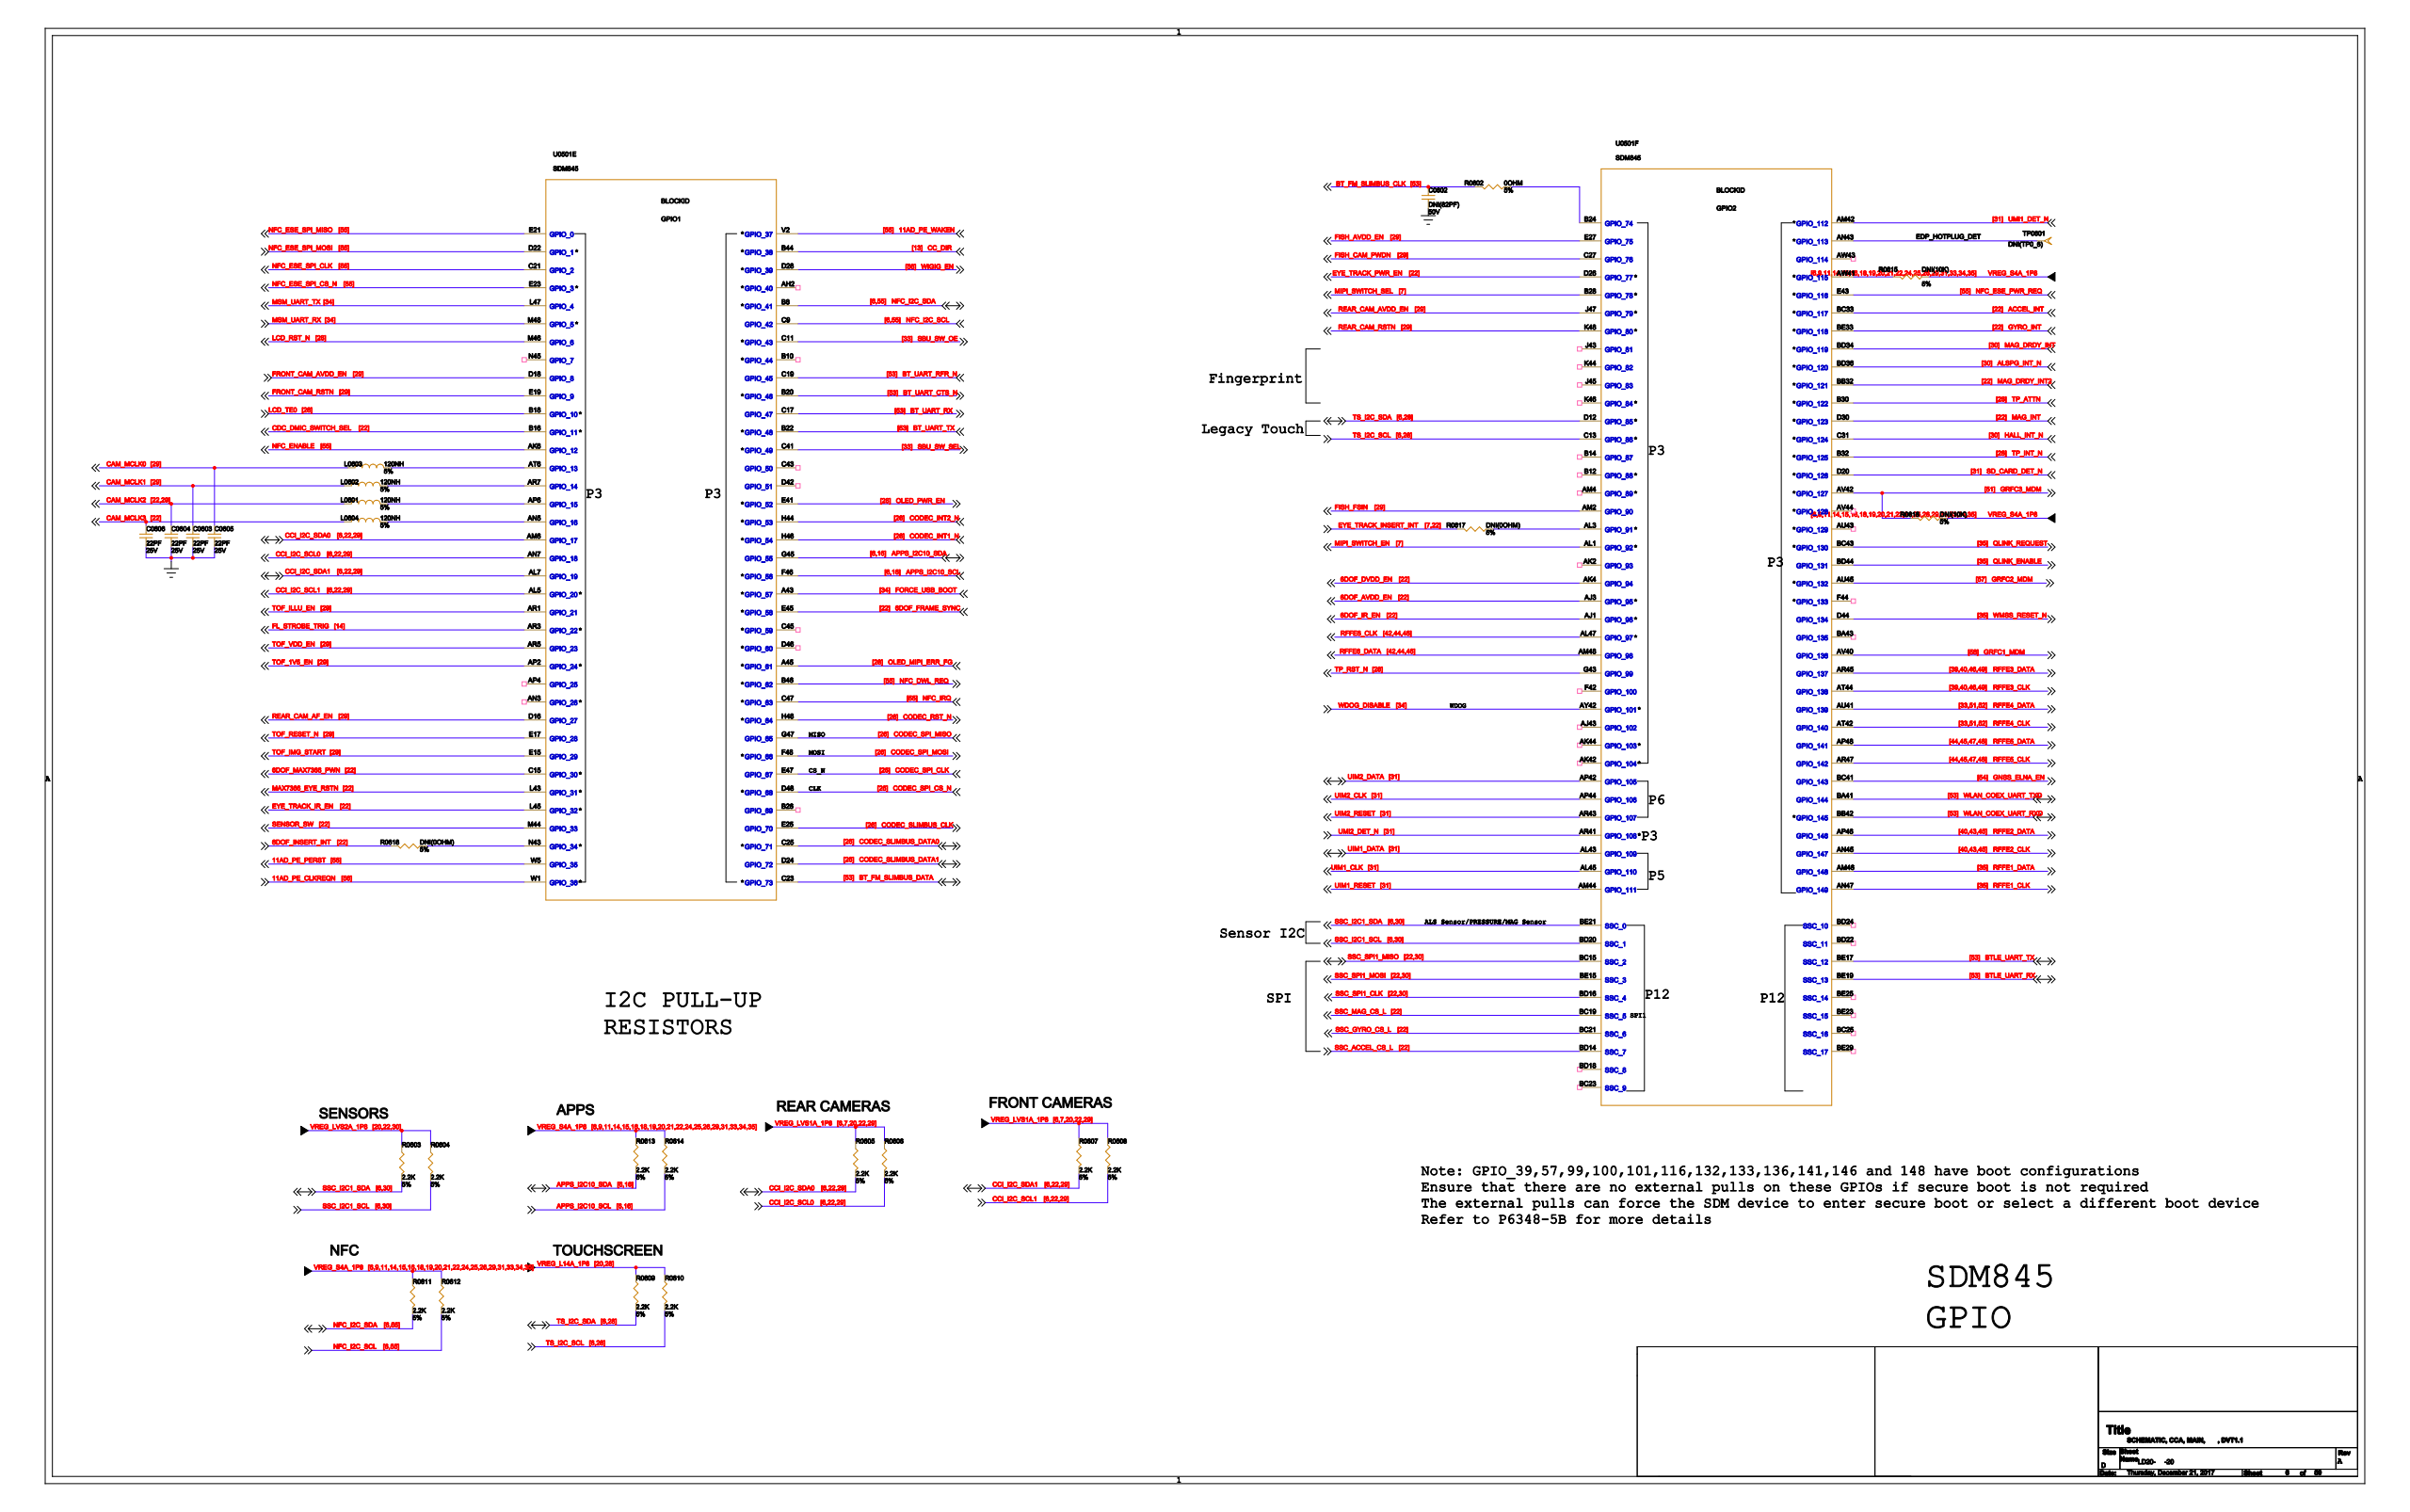Circuit board | Cadence Allegro | 1520 parts | 1149 nets | one sheet of the schematic
Parts on this sheet (reference | value | footprint):
C0602 | DNI(82PF) | 2P0201R_DNI
C0603 | 22PF | 2P0201R
C0604 | 22PF | 2P0201R
C0605 | 22PF | 2P0201R
C0606 | 22PF | 2P0201R
L0601 | 120NH | 2P0201R
L0602 | 120NH | 2P0201R
L0603 | 120NH | 2P0201R
L0604 | 120NH | 2P0201R
R0602 | 0OHM | 2P0201R
R0603 | 2.2K | 2P0201R
R0604 | 2.2K | 2P0201R
R0605 | 2.2K | 2P0201R
R0606 | 2.2K | 2P0201R
R0607 | 2.2K | 2P0201R
R0608 | 2.2K | 2P0201R
R0609 | 2.2K | 2P0201R
R0610 | 2.2K | 2P0201R
R0611 | 2.2K | 2P0201R
R0612 | 2.2K | 2P0201R
R0613 | 2.2K | 2P0201R
R0614 | 2.2K | 2P0201R
R0615 | DNI(10K) | 2P0201R_DNI
R0616 | DNI(10K) | 2P0201R_DNI
R0617 | DNI(0OHM) | 2P0201R_DNI
R0618 | DNI(0OHM) | 2P0201R_DNI
TP0601 | DNI(TP0_6) | TP-0_6
U0501 | SDM845 | 914PGA490X490B138D45
Nets of these parts (net: part-pin ...):
GND: C0602-2 C0603-2 C0604-2 C0605-2 C0606-2
VREG_S4A_1P8: R0611-2 R0612-2 R0613-2 R0614-2 R0615-2 R0616-2
ALSPG_INT_N: U0501-BD36
SSC_I2C1_SCL: R0604-1 U0501-BD20
SSC_I2C1_SDA: R0603-1 U0501-BE21
VREG_LVS2A_1P8: R0603-2 R0604-2
WIGIG_EN: U0501-D28
11AD_PE_CLKREQN: U0501-W1
11AD_PE_PERST: U0501-W5
11AD_PE_WAKEN: U0501-V2
RFFE2_CLK: U0501-AN45
RFFE5_CLK: U0501-AR47
RFFE2_DATA: U0501-AP46
RFFE5_DATA: U0501-AP48
CCI_I2C_SCL1: R0608-1 U0501-AL5
EYE_TRACK_INSERT_INT: R0617-1
CCI_I2C_SDA1: R0607-1 U0501-AL7
CAM_MCLK2: C0604-1 L0601-1
MAX7366_EYE_RSTN: U0501-L43
EYE_TRACK_PWR_EN: U0501-D26
EYE_TRACK_IR_EN: U0501-L45
6DOF_FRAME_SYNC: U0501-E45
6DOF_INSERT_INT: R0618-1
SSC_SPI1_MISO: U0501-BC15
SSC_SPI1_MOSI: U0501-BE15
SSC_SPI1_CLK: U0501-BD16
6DOF_IR_EN: U0501-AJ1
6DOF_AVDD_EN: U0501-AJ3
6DOF_DVDD_EN: U0501-AK4
VREG_LVS1A_1P8: R0605-2 R0606-2 R0607-2 R0608-2
CAM_MCLK1: C0603-1 L0602-1
6DOF_MAX7366_PWN: U0501-C15
CCI_I2C_SDA0: R0605-1 U0501-AM6
CCI_I2C_SCL0: R0606-1 U0501-AN7
VREG_L14A_1P8: R0609-2 R0610-2
BT_FM_SLIMBUS_CLK: C0602-1 R0602-1
SBU_SW_OE: U0501-C11
SBU_SW_SEL: U0501-C41
SSC_MAG_CS_L: U0501-BC19
SSC_ACCEL_CS_L: U0501-BD14
SSC_GYRO_CS_L: U0501-BC21
MAG_INT: U0501-D30
MAG_DRDY_INT2: U0501-BB32
ACCEL_INT: U0501-BC33
GYRO_INT: U0501-BE33
NFC_DWL_REQ: U0501-B46
NFC_ESE_SPI_MISO: U0501-E21
NFC_ESE_SPI_CLK: U0501-C21
NFC_ESE_SPI_CS_N: U0501-E23
NFC_ESE_SPI_MOSI: U0501-D22
NFC_I2C_SDA: R0611-1 U0501-B8
NFC_I2C_SCL: R0612-1 U0501-C9
NFC_IRQ: U0501-C47
NFC_ESE_PWR_REQ: U0501-E43
NFC_ENABLE: U0501-AK6
CODEC_INT1_N: U0501-H46
CODEC_INT2_N: U0501-H44
CODEC_RST_N: U0501-H48
CODEC_SLIMBUS_CLK: U0501-E25
CODEC_SLIMBUS_DATA0: U0501-C25
CODEC_SLIMBUS_DATA1: U0501-D24
CODEC_SPI_CLK: U0501-E47
CODEC_SPI_CS_N: U0501-D48
CODEC_SPI_MOSI: U0501-F48
CODEC_SPI_MISO: U0501-G47
BT_UART_RX: U0501-C17
LCD_TE0: U0501-B18
OLED_MIPI_ERR_FG: U0501-A45
TS_I2C_SDA: R0609-1 U0501-D12
TP_INT_N: U0501-B32
TP_RST_N: U0501-G43
TP_ATTN: U0501-B30
TS_I2C_SCL: R0610-1 U0501-C13
LCD_RST_N: U0501-M46
FORCE_USB_BOOT: U0501-A43
UIM2_CLK: U0501-AP44
UIM1_RESET: U0501-AM44
UIM1_CLK: U0501-AL45
UIM2_DATA: U0501-AP42
UIM1_DATA: U0501-AL43
UIM2_RESET: U0501-AR43
CAM_MCLK0: C0605-1 L0603-1
FRONT_CAM_AVDD_EN: U0501-D18
REAR_CAM_AVDD_EN: U0501-J47
REAR_CAM_AF_EN: U0501-D16
APPS_I2C10_SCL: R0614-1 U0501-F46
APPS_I2C10_SDA: R0613-1 U0501-G45
MAG_DRDY_INT: U0501-BD34
QLINK_ENABLE: U0501-BD44
QLINK_REQUEST: U0501-BC43
RFFE3_CLK: U0501-AT44
RFFE3_DATA: U0501-AR45
CAM_MCLK3: C0606-1 L0604-1
FRONT_CAM_RSTN: U0501-E19
GNSS_ELNA_EN: U0501-BC41
GRFC3_MDM: R0616-1 U0501-AV42
GRFC2_MDM: U0501-AU45
GRFC1_MDM: U0501-AV40
RFFE6_CLK: U0501-AL47
RFFE6_DATA: U0501-AM48
TOF_RESET_N: U0501-E17
FISH_CAM_PWDN: U0501-C27
TOF_IMG_START: U0501-E15
RFFE4_CLK: U0501-AT42
RFFE4_DATA: U0501-AU41
N49472447: R0602-2 U0501-B24
OLED_PWR_EN: U0501-E41
REAR_CAM_RSTN: U0501-K48
TOF_VDD_EN: U0501-AR5
TOF_1V5_EN: U0501-AP2
FISH_AVDD_EN: U0501-E27
FISH_FSIN: U0501-AM2
SD_CARD_DET_N: U0501-D20
UMI2_DET_N: U0501-AR41
UMI1_DET_N: U0501-AM42
WMSS_RESET_N: U0501-D44
RFFE1_CLK: U0501-AN47
RFFE1_DATA: U0501-AM46
TOF_ILLU_EN: U0501-AR1
MSM_UART_TX: U0501-L47
MSM_UART_RX: U0501-M48
WDOG_DISABLE: U0501-AY42
N49410165: L0604-2 U0501-AN5
N34902425: L0601-2 U0501-AP6
N34902416: L0602-2 U0501-AR7
N34902366: L0603-2 U0501-AT6
N37246227: R0615-1 U0501-AW41
N52367375: R0617-2 U0501-AL3
N52367399: R0618-2 U0501-N43
MIPI_SWITCH_SEL: U0501-B28
SENSOR_SW: U0501-M44
CDC_DMIC_SWITCH_SEL: U0501-B16
MIPI_SWITCH_EN: U0501-AL1
EDP_HOTPLUG_DET: TP0601-1 U0501-AN43
FL_STROBE_TRIG: U0501-AR3
CC_DIR: U0501-B44
BT_UART_RFR_N: U0501-C19
BT_UART_CTS_N: U0501-B20
BT_UART_TX: U0501-B22
BT_FM_SLIMBUS_DATA: U0501-C23
HALL_INT_N: U0501-C31
WLAN_COEX_UART_TXD: U0501-BA41
WLAN_COEX_UART_RXD: U0501-BB42
BTLE_UART_TX: U0501-BE17
BTLE_UART_RX: U0501-BE19